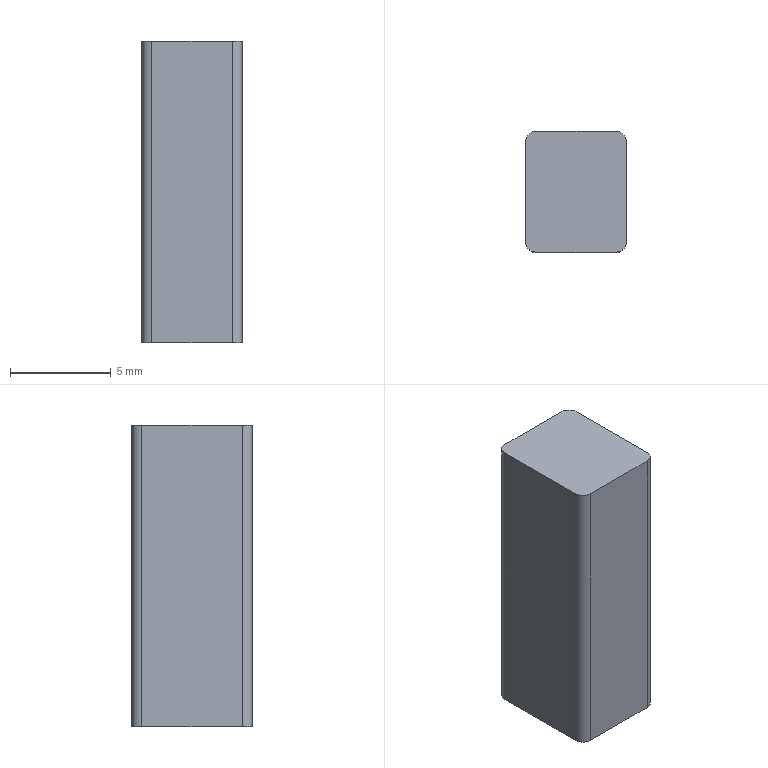Part | NX | features BREP 1 | 1 solid | 10 faces | box 5 x 6 x 15 mm | volume 446.781 mm3 | plane 6 | cylinder 4 | commonest cylinder face diameters 1 x4
STEP:
#1=CARTESIAN_POINT('',(-2.,3.,-25.6));
#2=VERTEX_POINT('',#1);
#3=CARTESIAN_POINT('',(-2.5,2.5,-25.6));
#4=VERTEX_POINT('',#3);
#5=CARTESIAN_POINT('',(-2.,2.5,-25.6));
#6=DIRECTION('',(0.,0.,1.));
#7=DIRECTION('',(1.,0.,0.));
#8=AXIS2_PLACEMENT_3D('',#5,#6,#7);
#9=CIRCLE('',#8,0.5);
#10=EDGE_CURVE('',#2,#4,#9,.T.);
#11=ORIENTED_EDGE('',*,*,#10,.F.);
#12=CARTESIAN_POINT('',(-2.,3.,-40.6));
#13=VERTEX_POINT('',#12);
#14=CARTESIAN_POINT('',(-2.,3.,-40.6));
#15=DIRECTION('',(0.,0.,1.));
#16=VECTOR('',#15,1000.);
#17=LINE('',#14,#16);
#18=EDGE_CURVE('',#13,#2,#17,.T.);
#19=ORIENTED_EDGE('',*,*,#18,.F.);
#20=CARTESIAN_POINT('',(-2.5,2.5,-40.6));
#21=VERTEX_POINT('',#20);
#22=CARTESIAN_POINT('',(-2.,2.5,-40.6));
#23=DIRECTION('',(0.,0.,1.));
#24=DIRECTION('',(1.,0.,0.));
#25=AXIS2_PLACEMENT_3D('',#22,#23,#24);
#26=CIRCLE('',#25,0.5);
#27=EDGE_CURVE('',#13,#21,#26,.T.);
#28=ORIENTED_EDGE('',*,*,#27,.T.);
#29=CARTESIAN_POINT('',(-2.5,2.5,-40.6));
#30=DIRECTION('',(0.,0.,1.));
#31=VECTOR('',#30,1000.);
#32=LINE('',#29,#31);
#33=EDGE_CURVE('',#21,#4,#32,.T.);
#34=ORIENTED_EDGE('',*,*,#33,.T.);
#35=EDGE_LOOP('',(#11,#19,#28,#34));
#36=FACE_BOUND('',#35,.T.);
#37=CARTESIAN_POINT('',(-2.,2.5,-40.6));
#38=DIRECTION('',(0.,0.,1.));
#39=DIRECTION('',(-1.,0.,0.));
#40=AXIS2_PLACEMENT_3D('',#37,#38,#39);
#41=CYLINDRICAL_SURFACE('',#40,0.5);
#42=ADVANCED_FACE('',(#36),#41,.T.);
#43=CARTESIAN_POINT('',(-2.5,-2.5,-25.6));
#44=VERTEX_POINT('',#43);
#45=CARTESIAN_POINT('',(-2.5,-2.5,-25.6));
#46=DIRECTION('',(0.,1.,0.));
#47=VECTOR('',#46,1000.);
#48=LINE('',#45,#47);
#49=EDGE_CURVE('',#44,#4,#48,.T.);
#50=ORIENTED_EDGE('',*,*,#49,.T.);
#51=ORIENTED_EDGE('',*,*,#33,.F.);
#52=CARTESIAN_POINT('',(-2.5,-2.5,-40.6));
#53=VERTEX_POINT('',#52);
#54=CARTESIAN_POINT('',(-2.5,-2.5,-40.6));
#55=DIRECTION('',(0.,1.,0.));
#56=VECTOR('',#55,1000.);
#57=LINE('',#54,#56);
#58=EDGE_CURVE('',#53,#21,#57,.T.);
#59=ORIENTED_EDGE('',*,*,#58,.F.);
#60=CARTESIAN_POINT('',(-2.5,-2.5,-40.6));
#61=DIRECTION('',(0.,0.,1.));
#62=VECTOR('',#61,1000.);
#63=LINE('',#60,#62);
#64=EDGE_CURVE('',#53,#44,#63,.T.);
#65=ORIENTED_EDGE('',*,*,#64,.T.);
#66=EDGE_LOOP('',(#50,#51,#59,#65));
#67=FACE_BOUND('',#66,.T.);
#68=CARTESIAN_POINT('',(-2.5,-2.5,-40.6));
#69=DIRECTION('',(1.,0.,0.));
#70=DIRECTION('',(0.,0.,1.));
#71=AXIS2_PLACEMENT_3D('',#68,#69,#70);
#72=PLANE('',#71);
#73=ADVANCED_FACE('',(#67),#72,.F.);
#74=CARTESIAN_POINT('',(-2.,-3.,-25.6));
#75=VERTEX_POINT('',#74);
#76=CARTESIAN_POINT('',(-2.,-2.5,-25.6));
#77=DIRECTION('',(0.,0.,1.));
#78=DIRECTION('',(1.,0.,0.));
#79=AXIS2_PLACEMENT_3D('',#76,#77,#78);
#80=CIRCLE('',#79,0.5);
#81=EDGE_CURVE('',#44,#75,#80,.T.);
#82=ORIENTED_EDGE('',*,*,#81,.F.);
#83=ORIENTED_EDGE('',*,*,#64,.F.);
#84=CARTESIAN_POINT('',(-2.,-3.,-40.6));
#85=VERTEX_POINT('',#84);
#86=CARTESIAN_POINT('',(-2.,-2.5,-40.6));
#87=DIRECTION('',(0.,0.,1.));
#88=DIRECTION('',(1.,0.,0.));
#89=AXIS2_PLACEMENT_3D('',#86,#87,#88);
#90=CIRCLE('',#89,0.5);
#91=EDGE_CURVE('',#53,#85,#90,.T.);
#92=ORIENTED_EDGE('',*,*,#91,.T.);
#93=CARTESIAN_POINT('',(-2.,-3.,-40.6));
#94=DIRECTION('',(0.,0.,1.));
#95=VECTOR('',#94,1000.);
#96=LINE('',#93,#95);
#97=EDGE_CURVE('',#85,#75,#96,.T.);
#98=ORIENTED_EDGE('',*,*,#97,.T.);
#99=EDGE_LOOP('',(#82,#83,#92,#98));
#100=FACE_BOUND('',#99,.T.);
#101=CARTESIAN_POINT('',(-2.,-2.5,-40.6));
#102=DIRECTION('',(0.,0.,1.));
#103=DIRECTION('',(-1.,0.,0.));
#104=AXIS2_PLACEMENT_3D('',#101,#102,#103);
#105=CYLINDRICAL_SURFACE('',#104,0.5);
#106=ADVANCED_FACE('',(#100),#105,.T.);
#107=CARTESIAN_POINT('',(2.,-3.,-25.6));
#108=VERTEX_POINT('',#107);
#109=CARTESIAN_POINT('',(2.,-3.,-25.6));
#110=DIRECTION('',(-1.,0.,0.));
#111=VECTOR('',#110,1000.);
#112=LINE('',#109,#111);
#113=EDGE_CURVE('',#108,#75,#112,.T.);
#114=ORIENTED_EDGE('',*,*,#113,.T.);
#115=ORIENTED_EDGE('',*,*,#97,.F.);
#116=CARTESIAN_POINT('',(2.,-3.,-40.6));
#117=VERTEX_POINT('',#116);
#118=CARTESIAN_POINT('',(2.,-3.,-40.6));
#119=DIRECTION('',(-1.,0.,0.));
#120=VECTOR('',#119,1000.);
#121=LINE('',#118,#120);
#122=EDGE_CURVE('',#117,#85,#121,.T.);
#123=ORIENTED_EDGE('',*,*,#122,.F.);
#124=CARTESIAN_POINT('',(2.,-3.,-40.6));
#125=DIRECTION('',(0.,0.,1.));
#126=VECTOR('',#125,1000.);
#127=LINE('',#124,#126);
#128=EDGE_CURVE('',#117,#108,#127,.T.);
#129=ORIENTED_EDGE('',*,*,#128,.T.);
#130=EDGE_LOOP('',(#114,#115,#123,#129));
#131=FACE_BOUND('',#130,.T.);
#132=CARTESIAN_POINT('',(2.,-3.,-40.6));
#133=DIRECTION('',(0.,1.,0.));
#134=DIRECTION('',(0.,0.,-1.));
#135=AXIS2_PLACEMENT_3D('',#132,#133,#134);
#136=PLANE('',#135);
#137=ADVANCED_FACE('',(#131),#136,.F.);
#138=CARTESIAN_POINT('',(2.5,-2.5,-25.6));
#139=VERTEX_POINT('',#138);
#140=CARTESIAN_POINT('',(2.,-2.5,-25.6));
#141=DIRECTION('',(0.,0.,1.));
#142=DIRECTION('',(1.,0.,0.));
#143=AXIS2_PLACEMENT_3D('',#140,#141,#142);
#144=CIRCLE('',#143,0.5);
#145=EDGE_CURVE('',#108,#139,#144,.T.);
#146=ORIENTED_EDGE('',*,*,#145,.F.);
#147=ORIENTED_EDGE('',*,*,#128,.F.);
#148=CARTESIAN_POINT('',(2.5,-2.5,-40.6));
#149=VERTEX_POINT('',#148);
#150=CARTESIAN_POINT('',(2.,-2.5,-40.6));
#151=DIRECTION('',(0.,0.,1.));
#152=DIRECTION('',(1.,0.,0.));
#153=AXIS2_PLACEMENT_3D('',#150,#151,#152);
#154=CIRCLE('',#153,0.5);
#155=EDGE_CURVE('',#117,#149,#154,.T.);
#156=ORIENTED_EDGE('',*,*,#155,.T.);
#157=CARTESIAN_POINT('',(2.5,-2.5,-40.6));
#158=DIRECTION('',(0.,0.,1.));
#159=VECTOR('',#158,1000.);
#160=LINE('',#157,#159);
#161=EDGE_CURVE('',#149,#139,#160,.T.);
#162=ORIENTED_EDGE('',*,*,#161,.T.);
#163=EDGE_LOOP('',(#146,#147,#156,#162));
#164=FACE_BOUND('',#163,.T.);
#165=CARTESIAN_POINT('',(2.,-2.5,-40.6));
#166=DIRECTION('',(0.,0.,1.));
#167=DIRECTION('',(-1.,0.,0.));
#168=AXIS2_PLACEMENT_3D('',#165,#166,#167);
#169=CYLINDRICAL_SURFACE('',#168,0.5);
#170=ADVANCED_FACE('',(#164),#169,.T.);
#171=CARTESIAN_POINT('',(2.5,2.5,-25.6));
#172=VERTEX_POINT('',#171);
#173=CARTESIAN_POINT('',(2.5,2.5,-25.6));
#174=DIRECTION('',(0.,-1.,0.));
#175=VECTOR('',#174,1000.);
#176=LINE('',#173,#175);
#177=EDGE_CURVE('',#172,#139,#176,.T.);
#178=ORIENTED_EDGE('',*,*,#177,.T.);
#179=ORIENTED_EDGE('',*,*,#161,.F.);
#180=CARTESIAN_POINT('',(2.5,2.5,-40.6));
#181=VERTEX_POINT('',#180);
#182=CARTESIAN_POINT('',(2.5,2.5,-40.6));
#183=DIRECTION('',(0.,-1.,0.));
#184=VECTOR('',#183,1000.);
#185=LINE('',#182,#184);
#186=EDGE_CURVE('',#181,#149,#185,.T.);
#187=ORIENTED_EDGE('',*,*,#186,.F.);
#188=CARTESIAN_POINT('',(2.5,2.5,-40.6));
#189=DIRECTION('',(0.,0.,1.));
#190=VECTOR('',#189,1000.);
#191=LINE('',#188,#190);
#192=EDGE_CURVE('',#181,#172,#191,.T.);
#193=ORIENTED_EDGE('',*,*,#192,.T.);
#194=EDGE_LOOP('',(#178,#179,#187,#193));
#195=FACE_BOUND('',#194,.T.);
#196=CARTESIAN_POINT('',(2.5,2.5,-40.6));
#197=DIRECTION('',(-1.,0.,0.));
#198=DIRECTION('',(0.,0.,-1.));
#199=AXIS2_PLACEMENT_3D('',#196,#197,#198);
#200=PLANE('',#199);
#201=ADVANCED_FACE('',(#195),#200,.F.);
#202=CARTESIAN_POINT('',(2.,3.,-25.6));
#203=VERTEX_POINT('',#202);
#204=CARTESIAN_POINT('',(2.,2.5,-25.6));
#205=DIRECTION('',(0.,0.,1.));
#206=DIRECTION('',(1.,0.,0.));
#207=AXIS2_PLACEMENT_3D('',#204,#205,#206);
#208=CIRCLE('',#207,0.5);
#209=EDGE_CURVE('',#172,#203,#208,.T.);
#210=ORIENTED_EDGE('',*,*,#209,.F.);
#211=ORIENTED_EDGE('',*,*,#192,.F.);
#212=CARTESIAN_POINT('',(2.,3.,-40.6));
#213=VERTEX_POINT('',#212);
#214=CARTESIAN_POINT('',(2.,2.5,-40.6));
#215=DIRECTION('',(0.,0.,1.));
#216=DIRECTION('',(1.,0.,0.));
#217=AXIS2_PLACEMENT_3D('',#214,#215,#216);
#218=CIRCLE('',#217,0.5);
#219=EDGE_CURVE('',#181,#213,#218,.T.);
#220=ORIENTED_EDGE('',*,*,#219,.T.);
#221=CARTESIAN_POINT('',(2.,3.,-40.6));
#222=DIRECTION('',(0.,0.,1.));
#223=VECTOR('',#222,1000.);
#224=LINE('',#221,#223);
#225=EDGE_CURVE('',#213,#203,#224,.T.);
#226=ORIENTED_EDGE('',*,*,#225,.T.);
#227=EDGE_LOOP('',(#210,#211,#220,#226));
#228=FACE_BOUND('',#227,.T.);
#229=CARTESIAN_POINT('',(2.,2.5,-40.6));
#230=DIRECTION('',(0.,0.,1.));
#231=DIRECTION('',(-1.,0.,0.));
#232=AXIS2_PLACEMENT_3D('',#229,#230,#231);
#233=CYLINDRICAL_SURFACE('',#232,0.5);
#234=ADVANCED_FACE('',(#228),#233,.T.);
#235=CARTESIAN_POINT('',(-2.,3.,-25.6));
#236=DIRECTION('',(1.,0.,0.));
#237=VECTOR('',#236,1000.);
#238=LINE('',#235,#237);
#239=EDGE_CURVE('',#2,#203,#238,.T.);
#240=ORIENTED_EDGE('',*,*,#239,.T.);
#241=ORIENTED_EDGE('',*,*,#225,.F.);
#242=CARTESIAN_POINT('',(-2.,3.,-40.6));
#243=DIRECTION('',(1.,0.,0.));
#244=VECTOR('',#243,1000.);
#245=LINE('',#242,#244);
#246=EDGE_CURVE('',#13,#213,#245,.T.);
#247=ORIENTED_EDGE('',*,*,#246,.F.);
#248=ORIENTED_EDGE('',*,*,#18,.T.);
#249=EDGE_LOOP('',(#240,#241,#247,#248));
#250=FACE_BOUND('',#249,.T.);
#251=CARTESIAN_POINT('',(-2.,3.,-40.6));
#252=DIRECTION('',(0.,-1.,0.));
#253=DIRECTION('',(0.,0.,1.));
#254=AXIS2_PLACEMENT_3D('',#251,#252,#253);
#255=PLANE('',#254);
#256=ADVANCED_FACE('',(#250),#255,.F.);
#257=ORIENTED_EDGE('',*,*,#27,.F.);
#258=ORIENTED_EDGE('',*,*,#246,.T.);
#259=ORIENTED_EDGE('',*,*,#219,.F.);
#260=ORIENTED_EDGE('',*,*,#186,.T.);
#261=ORIENTED_EDGE('',*,*,#155,.F.);
#262=ORIENTED_EDGE('',*,*,#122,.T.);
#263=ORIENTED_EDGE('',*,*,#91,.F.);
#264=ORIENTED_EDGE('',*,*,#58,.T.);
#265=EDGE_LOOP('',(#257,#258,#259,#260,#261,#262,#263,#264));
#266=FACE_BOUND('',#265,.T.);
#267=CARTESIAN_POINT('',(-2.,2.5,-40.6));
#268=DIRECTION('',(0.,0.,1.));
#269=DIRECTION('',(-1.,0.,0.));
#270=AXIS2_PLACEMENT_3D('',#267,#268,#269);
#271=PLANE('',#270);
#272=ADVANCED_FACE('',(#266),#271,.F.);
#273=ORIENTED_EDGE('',*,*,#10,.T.);
#274=ORIENTED_EDGE('',*,*,#49,.F.);
#275=ORIENTED_EDGE('',*,*,#81,.T.);
#276=ORIENTED_EDGE('',*,*,#113,.F.);
#277=ORIENTED_EDGE('',*,*,#145,.T.);
#278=ORIENTED_EDGE('',*,*,#177,.F.);
#279=ORIENTED_EDGE('',*,*,#209,.T.);
#280=ORIENTED_EDGE('',*,*,#239,.F.);
#281=EDGE_LOOP('',(#273,#274,#275,#276,#277,#278,#279,#280));
#282=FACE_BOUND('',#281,.T.);
#283=CARTESIAN_POINT('',(-2.,2.5,-25.6));
#284=DIRECTION('',(0.,0.,1.));
#285=DIRECTION('',(-1.,0.,0.));
#286=AXIS2_PLACEMENT_3D('',#283,#284,#285);
#287=PLANE('',#286);
#288=ADVANCED_FACE('',(#282),#287,.T.);
#289=CLOSED_SHELL('',(#42,#73,#106,#137,#170,#201,#234,#256,#272,#288));
#290=MANIFOLD_SOLID_BREP('',#289);
#291=(LENGTH_UNIT()NAMED_UNIT(*)SI_UNIT(.MILLI.,.METRE.));
#292=UNCERTAINTY_MEASURE_WITH_UNIT(LENGTH_MEASURE(0.00001),#291,'','');
#293=(NAMED_UNIT(*)PLANE_ANGLE_UNIT()SI_UNIT($,.RADIAN.));
#294=(NAMED_UNIT(*)SI_UNIT($,.STERADIAN.)SOLID_ANGLE_UNIT());
#295=(GEOMETRIC_REPRESENTATION_CONTEXT(3)GLOBAL_UNCERTAINTY_ASSIGNED_CONTEXT((#292))GLOBAL_UNIT_ASSIGNED_CONTEXT((#291,#293,#294))REPRESENTATION_CONTEXT('',''));
#296=ADVANCED_BREP_SHAPE_REPRESENTATION('',(#290),#295);